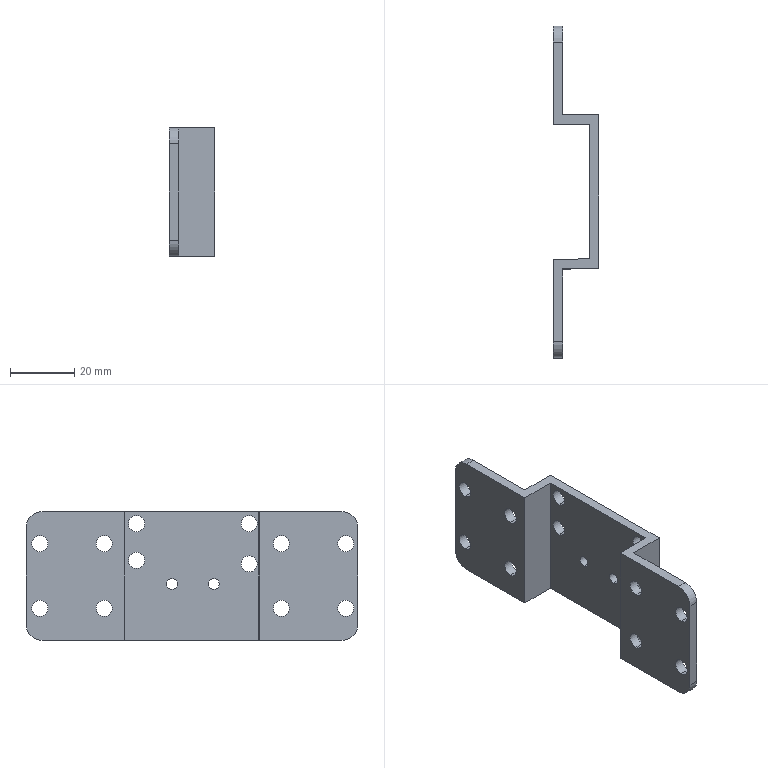Part | SolidWorks | features HoleWzd 2, ExtruThin 1, Fillet 1 | 1 solid | 46 faces | box 14.25 x 103.05 x 40 mm | volume 14217 mm3 | cylinder 32 | plane 14 | commonest cylinder face diameters 5 x24 3.4 x4 10 x4